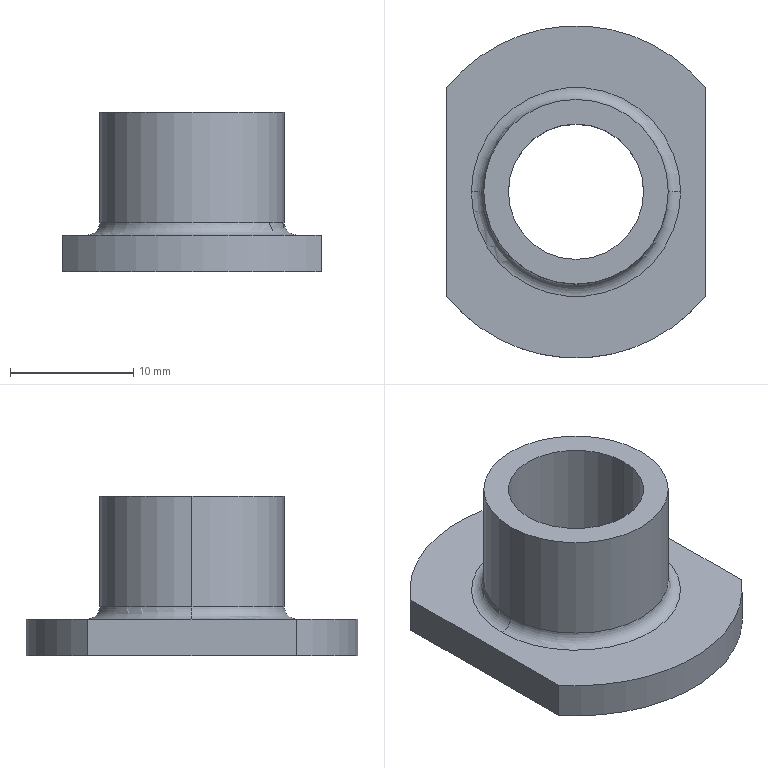Part | STEP file | FNA5401011 | 1 solid | 13 faces | box 21 x 27 x 13 mm | volume 2051 mm3 | cylinder 6 | plane 5 | torus 2 | commonest cylinder face diameters 11 x2 15 x2 27 x2
STEP:
#1=CARTESIAN_POINT('',(110.5,91.515,103.));
#2=VERTEX_POINT('',#1);
#3=CARTESIAN_POINT('',(110.5,108.485,103.));
#4=VERTEX_POINT('',#3);
#5=CARTESIAN_POINT('',(110.5,100.,103.));
#6=DIRECTION('',(0.,1.,0.));
#7=VECTOR('',#6,1.);
#8=LINE('',#5,#7);
#9=EDGE_CURVE('',#2,#4,#8,.T.);
#10=ORIENTED_EDGE('',*,*,#9,.F.);
#11=CARTESIAN_POINT('',(110.5,91.515,100.));
#12=VERTEX_POINT('',#11);
#13=CARTESIAN_POINT('',(110.5,91.515,101.5));
#14=DIRECTION('',(0.,0.,1.));
#15=VECTOR('',#14,1.);
#16=LINE('',#13,#15);
#17=EDGE_CURVE('',#12,#2,#16,.T.);
#18=ORIENTED_EDGE('',*,*,#17,.F.);
#19=CARTESIAN_POINT('',(110.5,108.485,100.));
#20=VERTEX_POINT('',#19);
#21=CARTESIAN_POINT('',(110.5,100.,100.));
#22=DIRECTION('',(0.,1.,0.));
#23=VECTOR('',#22,1.);
#24=LINE('',#21,#23);
#25=EDGE_CURVE('',#12,#20,#24,.T.);
#26=ORIENTED_EDGE('',*,*,#25,.T.);
#27=CARTESIAN_POINT('',(110.5,108.485,101.5));
#28=DIRECTION('',(0.,0.,1.));
#29=VECTOR('',#28,1.);
#30=LINE('',#27,#29);
#31=EDGE_CURVE('',#20,#4,#30,.T.);
#32=ORIENTED_EDGE('',*,*,#31,.T.);
#33=EDGE_LOOP('',(#10,#18,#26,#32));
#34=FACE_OUTER_BOUND('',#33,.T.);
#35=CARTESIAN_POINT('',(110.5,114.5,100.));
#36=DIRECTION('',(-1.,0.,0.));
#37=DIRECTION('',(0.,-1.,0.));
#38=AXIS2_PLACEMENT_3D('',#35,#36,#37);
#39=PLANE('',#38);
#40=ADVANCED_FACE('',(#34),#39,.F.);
#41=ORIENTED_EDGE('',*,*,#17,.T.);
#42=CARTESIAN_POINT('',(89.5,91.515,103.));
#43=VERTEX_POINT('',#42);
#44=CARTESIAN_POINT('',(100.,100.,103.));
#45=DIRECTION('',(0.,0.,1.));
#46=AXIS2_PLACEMENT_3D('',#44,#45,$);
#47=CIRCLE('',#46,13.5);
#48=EDGE_CURVE('',#43,#2,#47,.T.);
#49=ORIENTED_EDGE('',*,*,#48,.F.);
#50=CARTESIAN_POINT('',(89.5,91.515,100.));
#51=VERTEX_POINT('',#50);
#52=CARTESIAN_POINT('',(89.5,91.515,101.5));
#53=DIRECTION('',(0.,0.,1.));
#54=VECTOR('',#53,1.);
#55=LINE('',#52,#54);
#56=EDGE_CURVE('',#51,#43,#55,.T.);
#57=ORIENTED_EDGE('',*,*,#56,.F.);
#58=CARTESIAN_POINT('',(100.,100.,100.));
#59=DIRECTION('',(0.,0.,1.));
#60=AXIS2_PLACEMENT_3D('',#58,#59,$);
#61=CIRCLE('',#60,13.5);
#62=EDGE_CURVE('',#51,#12,#61,.T.);
#63=ORIENTED_EDGE('',*,*,#62,.T.);
#64=EDGE_LOOP('',(#41,#49,#57,#63));
#65=FACE_OUTER_BOUND('',#64,.T.);
#66=CARTESIAN_POINT('',(100.,100.,101.5));
#67=DIRECTION('',(0.,0.,1.));
#68=DIRECTION('',(1.,0.,0.));
#69=AXIS2_PLACEMENT_3D('',#66,#67,#68);
#70=CYLINDRICAL_SURFACE('',#69,13.5);
#71=ADVANCED_FACE('',(#65),#70,.T.);
#72=CARTESIAN_POINT('',(89.5,108.485,100.));
#73=VERTEX_POINT('',#72);
#74=CARTESIAN_POINT('',(89.5,108.485,103.));
#75=VERTEX_POINT('',#74);
#76=CARTESIAN_POINT('',(89.5,108.485,101.5));
#77=DIRECTION('',(0.,0.,1.));
#78=VECTOR('',#77,1.);
#79=LINE('',#76,#78);
#80=EDGE_CURVE('',#73,#75,#79,.T.);
#81=ORIENTED_EDGE('',*,*,#80,.F.);
#82=CARTESIAN_POINT('',(89.5,100.,100.));
#83=DIRECTION('',(0.,1.,0.));
#84=VECTOR('',#83,1.);
#85=LINE('',#82,#84);
#86=EDGE_CURVE('',#51,#73,#85,.T.);
#87=ORIENTED_EDGE('',*,*,#86,.F.);
#88=ORIENTED_EDGE('',*,*,#56,.T.);
#89=CARTESIAN_POINT('',(89.5,100.,103.));
#90=DIRECTION('',(0.,1.,0.));
#91=VECTOR('',#90,1.);
#92=LINE('',#89,#91);
#93=EDGE_CURVE('',#43,#75,#92,.T.);
#94=ORIENTED_EDGE('',*,*,#93,.T.);
#95=EDGE_LOOP('',(#81,#87,#88,#94));
#96=FACE_OUTER_BOUND('',#95,.T.);
#97=CARTESIAN_POINT('',(89.5,114.5,100.));
#98=DIRECTION('',(-1.,0.,0.));
#99=DIRECTION('',(0.,-1.,0.));
#100=AXIS2_PLACEMENT_3D('',#97,#98,#99);
#101=PLANE('',#100);
#102=ADVANCED_FACE('',(#96),#101,.T.);
#103=ORIENTED_EDGE('',*,*,#25,.F.);
#104=ORIENTED_EDGE('',*,*,#62,.F.);
#105=ORIENTED_EDGE('',*,*,#86,.T.);
#106=CARTESIAN_POINT('',(100.,100.,100.));
#107=DIRECTION('',(0.,0.,-1.));
#108=AXIS2_PLACEMENT_3D('',#106,#107,$);
#109=CIRCLE('',#108,13.5);
#110=EDGE_CURVE('',#20,#73,#109,.F.);
#111=ORIENTED_EDGE('',*,*,#110,.F.);
#112=EDGE_LOOP('',(#103,#104,#105,#111));
#113=FACE_OUTER_BOUND('',#112,.T.);
#114=CARTESIAN_POINT('',(94.5,100.,100.));
#115=VERTEX_POINT('',#114);
#116=CARTESIAN_POINT('',(105.5,100.,100.));
#117=VERTEX_POINT('',#116);
#118=CARTESIAN_POINT('',(100.,100.,100.));
#119=DIRECTION('',(0.,0.,-1.));
#120=AXIS2_PLACEMENT_3D('',#118,#119,$);
#121=CIRCLE('',#120,5.5);
#122=EDGE_CURVE('',#115,#117,#121,.T.);
#123=ORIENTED_EDGE('',*,*,#122,.F.);
#124=CARTESIAN_POINT('',(100.,100.,100.));
#125=DIRECTION('',(0.,0.,-1.));
#126=AXIS2_PLACEMENT_3D('',#124,#125,$);
#127=CIRCLE('',#126,5.5);
#128=EDGE_CURVE('',#117,#115,#127,.T.);
#129=ORIENTED_EDGE('',*,*,#128,.F.);
#130=EDGE_LOOP('',(#123,#129));
#131=FACE_BOUND('',#130,.T.);
#132=CARTESIAN_POINT('',(100.,106.372,100.));
#133=DIRECTION('',(0.,0.,-1.));
#134=DIRECTION('',(1.,-0.000006639,0.));
#135=AXIS2_PLACEMENT_3D('',#132,#133,#134);
#136=PLANE('',#135);
#137=ADVANCED_FACE('',(#113,#131),#136,.T.);
#138=ORIENTED_EDGE('',*,*,#122,.T.);
#139=CARTESIAN_POINT('',(105.5,100.,113.));
#140=VERTEX_POINT('',#139);
#141=CARTESIAN_POINT('',(105.5,100.,106.5));
#142=DIRECTION('',(0.,0.,1.));
#143=VECTOR('',#142,1.);
#144=LINE('',#141,#143);
#145=EDGE_CURVE('',#117,#140,#144,.T.);
#146=ORIENTED_EDGE('',*,*,#145,.T.);
#147=CARTESIAN_POINT('',(94.5,100.,113.));
#148=VERTEX_POINT('',#147);
#149=CARTESIAN_POINT('',(100.,100.,113.));
#150=DIRECTION('',(0.,0.,1.));
#151=AXIS2_PLACEMENT_3D('',#149,#150,$);
#152=CIRCLE('',#151,5.5);
#153=EDGE_CURVE('',#148,#140,#152,.F.);
#154=ORIENTED_EDGE('',*,*,#153,.F.);
#155=CARTESIAN_POINT('',(94.5,100.,106.5));
#156=DIRECTION('',(0.,0.,1.));
#157=VECTOR('',#156,1.);
#158=LINE('',#155,#157);
#159=EDGE_CURVE('',#115,#148,#158,.T.);
#160=ORIENTED_EDGE('',*,*,#159,.F.);
#161=EDGE_LOOP('',(#138,#146,#154,#160));
#162=FACE_OUTER_BOUND('',#161,.T.);
#163=CARTESIAN_POINT('',(100.,100.,105.));
#164=DIRECTION('',(0.,0.,1.));
#165=DIRECTION('',(1.,0.,0.));
#166=AXIS2_PLACEMENT_3D('',#163,#164,#165);
#167=CYLINDRICAL_SURFACE('',#166,5.5);
#168=ADVANCED_FACE('',(#162),#167,.F.);
#169=CARTESIAN_POINT('',(92.5,100.,113.));
#170=VERTEX_POINT('',#169);
#171=CARTESIAN_POINT('',(107.5,100.,113.));
#172=VERTEX_POINT('',#171);
#173=CARTESIAN_POINT('',(100.,100.,113.));
#174=DIRECTION('',(0.,0.,-1.));
#175=AXIS2_PLACEMENT_3D('',#173,#174,$);
#176=CIRCLE('',#175,7.5);
#177=EDGE_CURVE('',#170,#172,#176,.F.);
#178=ORIENTED_EDGE('',*,*,#177,.T.);
#179=CARTESIAN_POINT('',(100.,100.,113.));
#180=DIRECTION('',(0.,0.,-1.));
#181=AXIS2_PLACEMENT_3D('',#179,#180,$);
#182=CIRCLE('',#181,7.5);
#183=EDGE_CURVE('',#172,#170,#182,.F.);
#184=ORIENTED_EDGE('',*,*,#183,.T.);
#185=EDGE_LOOP('',(#178,#184));
#186=FACE_OUTER_BOUND('',#185,.T.);
#187=CARTESIAN_POINT('',(100.,100.,113.));
#188=DIRECTION('',(0.,0.,-1.));
#189=AXIS2_PLACEMENT_3D('',#187,#188,$);
#190=CIRCLE('',#189,5.5);
#191=EDGE_CURVE('',#140,#148,#190,.T.);
#192=ORIENTED_EDGE('',*,*,#191,.T.);
#193=ORIENTED_EDGE('',*,*,#153,.T.);
#194=EDGE_LOOP('',(#192,#193));
#195=FACE_BOUND('',#194,.T.);
#196=CARTESIAN_POINT('',(100.,103.54,113.));
#197=DIRECTION('',(0.,0.,-1.));
#198=DIRECTION('',(1.,-0.000006639,0.));
#199=AXIS2_PLACEMENT_3D('',#196,#197,#198);
#200=PLANE('',#199);
#201=ADVANCED_FACE('',(#186,#195),#200,.F.);
#202=CARTESIAN_POINT('',(92.5,100.,104.));
#203=VERTEX_POINT('',#202);
#204=CARTESIAN_POINT('',(92.5,100.,107.5));
#205=DIRECTION('',(0.,0.,1.));
#206=VECTOR('',#205,1.);
#207=LINE('',#204,#206);
#208=EDGE_CURVE('',#203,#170,#207,.T.);
#209=ORIENTED_EDGE('',*,*,#208,.T.);
#210=ORIENTED_EDGE('',*,*,#183,.F.);
#211=CARTESIAN_POINT('',(107.5,100.,104.));
#212=VERTEX_POINT('',#211);
#213=CARTESIAN_POINT('',(107.5,100.,107.5));
#214=DIRECTION('',(0.,0.,1.));
#215=VECTOR('',#214,1.);
#216=LINE('',#213,#215);
#217=EDGE_CURVE('',#212,#172,#216,.T.);
#218=ORIENTED_EDGE('',*,*,#217,.F.);
#219=CARTESIAN_POINT('',(100.,100.,104.));
#220=DIRECTION('',(0.,0.,1.));
#221=AXIS2_PLACEMENT_3D('',#219,#220,$);
#222=CIRCLE('',#221,7.5);
#223=EDGE_CURVE('',#212,#203,#222,.T.);
#224=ORIENTED_EDGE('',*,*,#223,.T.);
#225=EDGE_LOOP('',(#209,#210,#218,#224));
#226=FACE_OUTER_BOUND('',#225,.T.);
#227=CARTESIAN_POINT('',(100.,100.,107.5));
#228=DIRECTION('',(0.,0.,1.));
#229=DIRECTION('',(1.,0.,0.));
#230=AXIS2_PLACEMENT_3D('',#227,#228,#229);
#231=CYLINDRICAL_SURFACE('',#230,7.5);
#232=ADVANCED_FACE('',(#226),#231,.T.);
#233=CARTESIAN_POINT('',(108.5,100.,103.));
#234=VERTEX_POINT('',#233);
#235=CARTESIAN_POINT('',(91.5,100.,103.));
#236=VERTEX_POINT('',#235);
#237=CARTESIAN_POINT('',(100.,100.,103.));
#238=DIRECTION('',(0.,0.,-1.));
#239=AXIS2_PLACEMENT_3D('',#237,#238,$);
#240=CIRCLE('',#239,8.5);
#241=EDGE_CURVE('',#234,#236,#240,.F.);
#242=ORIENTED_EDGE('',*,*,#241,.T.);
#243=CARTESIAN_POINT('',(91.5,100.,104.));
#244=DIRECTION('',(0.,-1.,0.));
#245=AXIS2_PLACEMENT_3D('',#243,#244,$);
#246=CIRCLE('',#245,1.);
#247=EDGE_CURVE('',#236,#203,#246,.T.);
#248=ORIENTED_EDGE('',*,*,#247,.T.);
#249=ORIENTED_EDGE('',*,*,#223,.F.);
#250=CARTESIAN_POINT('',(108.5,100.,104.));
#251=DIRECTION('',(0.,1.,0.));
#252=AXIS2_PLACEMENT_3D('',#250,#251,$);
#253=CIRCLE('',#252,1.);
#254=EDGE_CURVE('',#234,#212,#253,.T.);
#255=ORIENTED_EDGE('',*,*,#254,.F.);
#256=EDGE_LOOP('',(#242,#248,#249,#255));
#257=FACE_OUTER_BOUND('',#256,.T.);
#258=CARTESIAN_POINT('',(100.,100.,104.));
#259=DIRECTION('',(0.,0.,-1.));
#260=DIRECTION('',(-0.9832,-0.1826,0.));
#261=AXIS2_PLACEMENT_3D('',#258,#259,#260);
#262=TOROIDAL_SURFACE('',#261,8.5,1.);
#263=ADVANCED_FACE('',(#257),#262,.F.);
#264=CARTESIAN_POINT('',(100.,100.,103.));
#265=DIRECTION('',(0.,0.,-1.));
#266=AXIS2_PLACEMENT_3D('',#264,#265,$);
#267=CIRCLE('',#266,13.5);
#268=EDGE_CURVE('',#4,#75,#267,.F.);
#269=ORIENTED_EDGE('',*,*,#268,.T.);
#270=ORIENTED_EDGE('',*,*,#93,.F.);
#271=ORIENTED_EDGE('',*,*,#48,.T.);
#272=ORIENTED_EDGE('',*,*,#9,.T.);
#273=EDGE_LOOP('',(#269,#270,#271,#272));
#274=FACE_OUTER_BOUND('',#273,.T.);
#275=ORIENTED_EDGE('',*,*,#241,.F.);
#276=CARTESIAN_POINT('',(100.,100.,103.));
#277=DIRECTION('',(0.,0.,-1.));
#278=AXIS2_PLACEMENT_3D('',#276,#277,$);
#279=CIRCLE('',#278,8.5);
#280=EDGE_CURVE('',#236,#234,#279,.F.);
#281=ORIENTED_EDGE('',*,*,#280,.F.);
#282=EDGE_LOOP('',(#275,#281));
#283=FACE_BOUND('',#282,.T.);
#284=CARTESIAN_POINT('',(100.,106.372,103.));
#285=DIRECTION('',(0.,0.,-1.));
#286=DIRECTION('',(1.,-0.000006639,0.));
#287=AXIS2_PLACEMENT_3D('',#284,#285,#286);
#288=PLANE('',#287);
#289=ADVANCED_FACE('',(#274,#283),#288,.F.);
#290=ORIENTED_EDGE('',*,*,#80,.T.);
#291=ORIENTED_EDGE('',*,*,#268,.F.);
#292=ORIENTED_EDGE('',*,*,#31,.F.);
#293=ORIENTED_EDGE('',*,*,#110,.T.);
#294=EDGE_LOOP('',(#290,#291,#292,#293));
#295=FACE_OUTER_BOUND('',#294,.T.);
#296=ADVANCED_FACE('',(#295),#70,.T.);
#297=ORIENTED_EDGE('',*,*,#159,.T.);
#298=ORIENTED_EDGE('',*,*,#191,.F.);
#299=ORIENTED_EDGE('',*,*,#145,.F.);
#300=ORIENTED_EDGE('',*,*,#128,.T.);
#301=EDGE_LOOP('',(#297,#298,#299,#300));
#302=FACE_OUTER_BOUND('',#301,.T.);
#303=ADVANCED_FACE('',(#302),#167,.F.);
#304=ORIENTED_EDGE('',*,*,#280,.T.);
#305=ORIENTED_EDGE('',*,*,#254,.T.);
#306=CARTESIAN_POINT('',(100.,100.,104.));
#307=DIRECTION('',(0.,0.,-1.));
#308=AXIS2_PLACEMENT_3D('',#306,#307,$);
#309=CIRCLE('',#308,7.5);
#310=EDGE_CURVE('',#203,#212,#309,.F.);
#311=ORIENTED_EDGE('',*,*,#310,.F.);
#312=ORIENTED_EDGE('',*,*,#247,.F.);
#313=EDGE_LOOP('',(#304,#305,#311,#312));
#314=FACE_OUTER_BOUND('',#313,.T.);
#315=CARTESIAN_POINT('',(100.,100.,104.));
#316=DIRECTION('',(0.,0.,-1.));
#317=DIRECTION('',(1.,0.,0.));
#318=AXIS2_PLACEMENT_3D('',#315,#316,#317);
#319=TOROIDAL_SURFACE('',#318,8.5,1.);
#320=ADVANCED_FACE('',(#314),#319,.F.);
#321=ORIENTED_EDGE('',*,*,#217,.T.);
#322=ORIENTED_EDGE('',*,*,#177,.F.);
#323=ORIENTED_EDGE('',*,*,#208,.F.);
#324=ORIENTED_EDGE('',*,*,#310,.T.);
#325=EDGE_LOOP('',(#321,#322,#323,#324));
#326=FACE_OUTER_BOUND('',#325,.T.);
#327=ADVANCED_FACE('',(#326),#231,.T.);
#328=CLOSED_SHELL('',(#40,#71,#102,#137,#168,#201,#232,#263,#289,#296,#303,#320,#327));
#329=MANIFOLD_SOLID_BREP('',#328);
#330=(LENGTH_UNIT()NAMED_UNIT(*)SI_UNIT(.MILLI.,.METRE.));
#331=UNCERTAINTY_MEASURE_WITH_UNIT(LENGTH_MEASURE(0.005),#330,'','');
#332=(NAMED_UNIT(*)PLANE_ANGLE_UNIT()SI_UNIT($,.RADIAN.));
#333=(NAMED_UNIT(*)SI_UNIT($,.STERADIAN.)SOLID_ANGLE_UNIT());
#334=(GEOMETRIC_REPRESENTATION_CONTEXT(3)GLOBAL_UNCERTAINTY_ASSIGNED_CONTEXT((#331))GLOBAL_UNIT_ASSIGNED_CONTEXT((#330,#332,#333))REPRESENTATION_CONTEXT('',''));
#335=ADVANCED_BREP_SHAPE_REPRESENTATION('',(#329),#334);